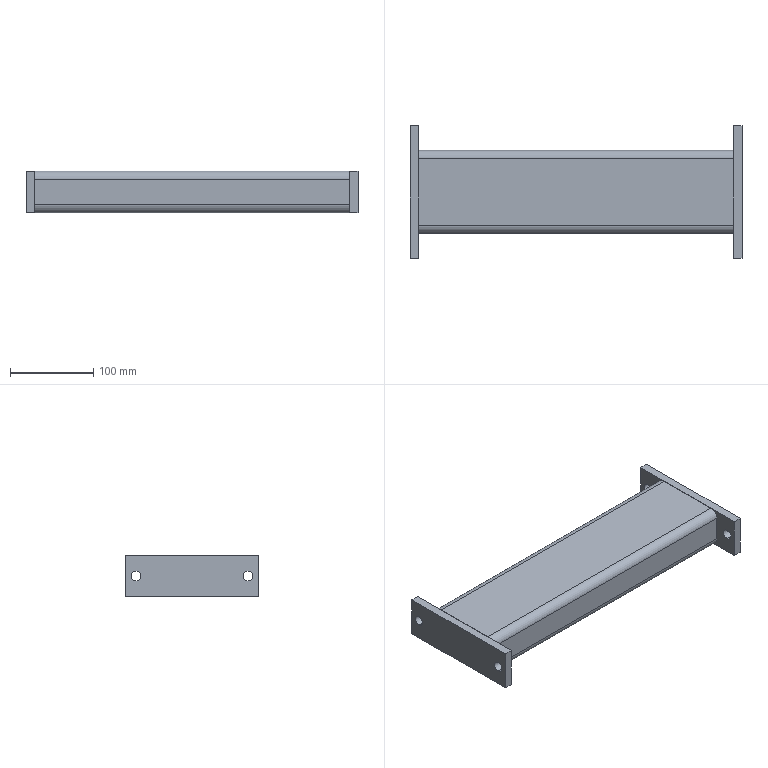Part | STEP file | PN_0010_cross beam_default_machined_ | 3 solids | 38 faces | box 400 x 160 x 50 mm | volume 663011 mm3 | plane 22 | cylinder 16 | commonest cylinder face diameters 12 x8 10 x4 20 x4